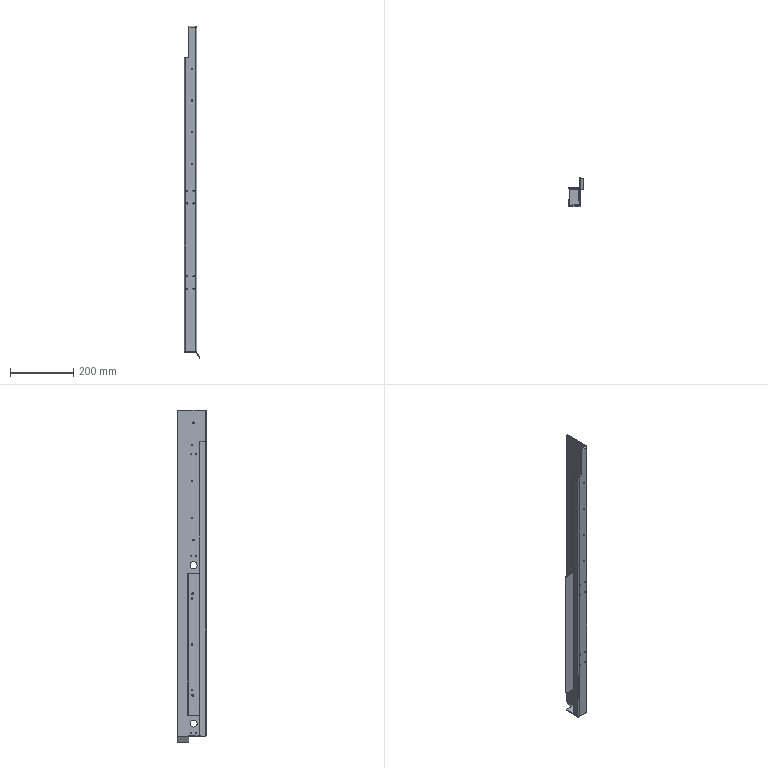Part | SolidWorks | features HoleWzd 13, EdgeFlange 6, ICE 4, Fillet 2, FlatPattern 2, SMBaseFlange 2, SheetMetal 2 | 2 solids | 135 faces | box 49.598 x 90 x 1048 mm | volume 529976 mm3 | cylinder 85 | plane 50 | commonest cylinder face diameters 4.2 x30 3.2 x18 6.5 x8 0.8 x6 3.3 x6 6.8 x6